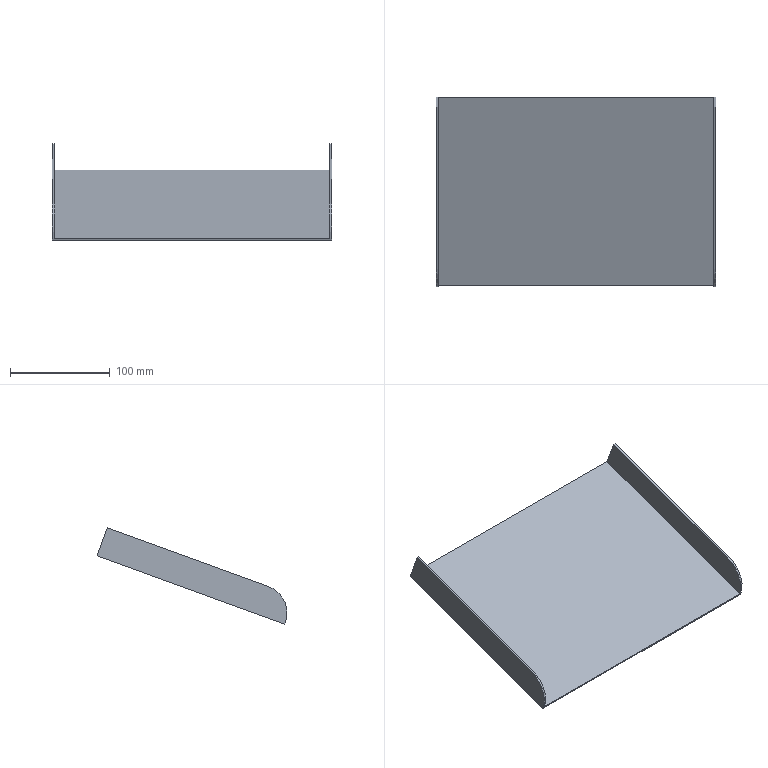Part | NX | features solid 2 | 1 solid | 12 faces | box 280.45 x 190.311 x 96.595 mm | volume 133907 mm3 | plane 10 | cylinder 2 | commonest cylinder face diameters 56 x2
STEP:
#1=CARTESIAN_POINT('',(-293.45,-997.939,-367.986));
#2=VERTEX_POINT('',#1);
#3=CARTESIAN_POINT('',(-17.,-997.939,-367.986));
#4=VERTEX_POINT('',#3);
#5=CARTESIAN_POINT('',(-283.45,-997.939,-367.986));
#6=DIRECTION('',(1.,0.,0.));
#7=VECTOR('',#6,1000.);
#8=LINE('',#5,#7);
#9=EDGE_CURVE('',#2,#4,#8,.T.);
#10=ORIENTED_EDGE('',*,*,#9,.T.);
#11=CARTESIAN_POINT('',(-17.,-810.,-299.582));
#12=VERTEX_POINT('',#11);
#13=CARTESIAN_POINT('',(-17.,-838.191,-309.843));
#14=DIRECTION('',(0.,0.9397,0.342));
#15=VECTOR('',#14,1000.);
#16=LINE('',#13,#15);
#17=EDGE_CURVE('',#4,#12,#16,.T.);
#18=ORIENTED_EDGE('',*,*,#17,.T.);
#19=CARTESIAN_POINT('',(-293.45,-810.,-299.582));
#20=VERTEX_POINT('',#19);
#21=CARTESIAN_POINT('',(-283.45,-810.,-299.582));
#22=DIRECTION('',(1.,0.,0.));
#23=VECTOR('',#22,1000.);
#24=LINE('',#21,#23);
#25=EDGE_CURVE('',#20,#12,#24,.T.);
#26=ORIENTED_EDGE('',*,*,#25,.F.);
#27=CARTESIAN_POINT('',(-293.45,-838.191,-309.843));
#28=DIRECTION('',(0.,0.9397,0.342));
#29=VECTOR('',#28,1000.);
#30=LINE('',#27,#29);
#31=EDGE_CURVE('',#2,#20,#30,.T.);
#32=ORIENTED_EDGE('',*,*,#31,.F.);
#33=EDGE_LOOP('',(#10,#18,#26,#32));
#34=FACE_BOUND('',#33,.T.);
#35=CARTESIAN_POINT('',(-283.45,-838.191,-309.843));
#36=DIRECTION('',(0.,0.342,-0.9397));
#37=DIRECTION('',(-1.,0.,0.));
#38=AXIS2_PLACEMENT_3D('',#35,#36,#37);
#39=PLANE('',#38);
#40=ADVANCED_FACE('',(#34),#39,.F.);
#41=CARTESIAN_POINT('',(-295.45,-997.254,-369.866));
#42=VERTEX_POINT('',#41);
#43=CARTESIAN_POINT('',(-15.,-997.254,-369.866));
#44=VERTEX_POINT('',#43);
#45=CARTESIAN_POINT('',(-283.45,-997.254,-369.866));
#46=DIRECTION('',(1.,0.,0.));
#47=VECTOR('',#46,1000.);
#48=LINE('',#45,#47);
#49=EDGE_CURVE('',#42,#44,#48,.T.);
#50=ORIENTED_EDGE('',*,*,#49,.T.);
#51=CARTESIAN_POINT('',(-15.,-997.939,-367.986));
#52=VERTEX_POINT('',#51);
#53=CARTESIAN_POINT('',(-15.,-997.254,-369.866));
#54=DIRECTION('',(0.,-0.342,0.9397));
#55=VECTOR('',#54,1000.);
#56=LINE('',#53,#55);
#57=EDGE_CURVE('',#44,#52,#56,.T.);
#58=ORIENTED_EDGE('',*,*,#57,.T.);
#59=CARTESIAN_POINT('',(-15.,-997.939,-367.986));
#60=DIRECTION('',(-1.,0.,0.));
#61=VECTOR('',#60,1000.);
#62=LINE('',#59,#61);
#63=EDGE_CURVE('',#52,#4,#62,.T.);
#64=ORIENTED_EDGE('',*,*,#63,.T.);
#65=ORIENTED_EDGE('',*,*,#9,.F.);
#66=CARTESIAN_POINT('',(-295.45,-997.939,-367.986));
#67=VERTEX_POINT('',#66);
#68=CARTESIAN_POINT('',(-283.45,-997.939,-367.986));
#69=DIRECTION('',(1.,0.,0.));
#70=VECTOR('',#69,1000.);
#71=LINE('',#68,#70);
#72=EDGE_CURVE('',#67,#2,#71,.T.);
#73=ORIENTED_EDGE('',*,*,#72,.F.);
#74=CARTESIAN_POINT('',(-295.45,-997.254,-369.866));
#75=DIRECTION('',(0.,-0.342,0.9397));
#76=VECTOR('',#75,1000.);
#77=LINE('',#74,#76);
#78=EDGE_CURVE('',#42,#67,#77,.T.);
#79=ORIENTED_EDGE('',*,*,#78,.F.);
#80=EDGE_LOOP('',(#50,#58,#64,#65,#73,#79));
#81=FACE_BOUND('',#80,.T.);
#82=CARTESIAN_POINT('',(-283.45,-997.254,-369.866));
#83=DIRECTION('',(0.,-0.9397,-0.342));
#84=DIRECTION('',(0.,0.342,-0.9397));
#85=AXIS2_PLACEMENT_3D('',#82,#83,#84);
#86=PLANE('',#85);
#87=ADVANCED_FACE('',(#81),#86,.T.);
#88=ORIENTED_EDGE('',*,*,#78,.T.);
#89=CARTESIAN_POINT('',(-295.45,-981.204,-332.098));
#90=VERTEX_POINT('',#89);
#91=CARTESIAN_POINT('',(-295.45,-971.627,-358.41));
#92=DIRECTION('',(-1.,0.,0.));
#93=DIRECTION('',(0.,0.,1.));
#94=AXIS2_PLACEMENT_3D('',#91,#92,#93);
#95=CIRCLE('',#94,28.);
#96=EDGE_CURVE('',#67,#90,#95,.T.);
#97=ORIENTED_EDGE('',*,*,#96,.T.);
#98=CARTESIAN_POINT('',(-295.45,-819.577,-273.271));
#99=VERTEX_POINT('',#98);
#100=CARTESIAN_POINT('',(-295.45,-819.577,-273.271));
#101=DIRECTION('',(0.,-0.9397,-0.342));
#102=VECTOR('',#101,1000.);
#103=LINE('',#100,#102);
#104=EDGE_CURVE('',#99,#90,#103,.T.);
#105=ORIENTED_EDGE('',*,*,#104,.F.);
#106=CARTESIAN_POINT('',(-295.45,-809.316,-301.462));
#107=VERTEX_POINT('',#106);
#108=CARTESIAN_POINT('',(-295.45,-809.316,-301.462));
#109=DIRECTION('',(0.,-0.342,0.9397));
#110=VECTOR('',#109,1000.);
#111=LINE('',#108,#110);
#112=EDGE_CURVE('',#107,#99,#111,.T.);
#113=ORIENTED_EDGE('',*,*,#112,.F.);
#114=CARTESIAN_POINT('',(-295.45,-837.507,-311.722));
#115=DIRECTION('',(0.,-0.9397,-0.342));
#116=VECTOR('',#115,1000.);
#117=LINE('',#114,#116);
#118=EDGE_CURVE('',#107,#42,#117,.T.);
#119=ORIENTED_EDGE('',*,*,#118,.T.);
#120=EDGE_LOOP('',(#88,#97,#105,#113,#119));
#121=FACE_BOUND('',#120,.T.);
#122=CARTESIAN_POINT('',(-295.45,-837.507,-311.722));
#123=DIRECTION('',(-1.,0.,0.));
#124=DIRECTION('',(0.,-0.342,0.9397));
#125=AXIS2_PLACEMENT_3D('',#122,#123,#124);
#126=PLANE('',#125);
#127=ADVANCED_FACE('',(#121),#126,.T.);
#128=ORIENTED_EDGE('',*,*,#25,.T.);
#129=CARTESIAN_POINT('',(-17.,-819.577,-273.271));
#130=VERTEX_POINT('',#129);
#131=CARTESIAN_POINT('',(-17.,-809.316,-301.462));
#132=DIRECTION('',(0.,-0.342,0.9397));
#133=VECTOR('',#132,1000.);
#134=LINE('',#131,#133);
#135=EDGE_CURVE('',#12,#130,#134,.T.);
#136=ORIENTED_EDGE('',*,*,#135,.T.);
#137=CARTESIAN_POINT('',(-15.,-819.577,-273.271));
#138=VERTEX_POINT('',#137);
#139=CARTESIAN_POINT('',(-15.,-819.577,-273.271));
#140=DIRECTION('',(1.,0.,0.));
#141=VECTOR('',#140,1000.);
#142=LINE('',#139,#141);
#143=EDGE_CURVE('',#138,#130,#142,.F.);
#144=ORIENTED_EDGE('',*,*,#143,.F.);
#145=CARTESIAN_POINT('',(-15.,-809.316,-301.462));
#146=VERTEX_POINT('',#145);
#147=CARTESIAN_POINT('',(-15.,-809.316,-301.462));
#148=DIRECTION('',(0.,-0.342,0.9397));
#149=VECTOR('',#148,1000.);
#150=LINE('',#147,#149);
#151=EDGE_CURVE('',#146,#138,#150,.T.);
#152=ORIENTED_EDGE('',*,*,#151,.F.);
#153=CARTESIAN_POINT('',(-283.45,-809.316,-301.462));
#154=DIRECTION('',(1.,0.,0.));
#155=VECTOR('',#154,1000.);
#156=LINE('',#153,#155);
#157=EDGE_CURVE('',#107,#146,#156,.T.);
#158=ORIENTED_EDGE('',*,*,#157,.F.);
#159=ORIENTED_EDGE('',*,*,#112,.T.);
#160=CARTESIAN_POINT('',(-293.45,-819.577,-273.271));
#161=VERTEX_POINT('',#160);
#162=CARTESIAN_POINT('',(-295.45,-819.577,-273.271));
#163=DIRECTION('',(1.,0.,0.));
#164=VECTOR('',#163,1000.);
#165=LINE('',#162,#164);
#166=EDGE_CURVE('',#99,#161,#165,.T.);
#167=ORIENTED_EDGE('',*,*,#166,.T.);
#168=CARTESIAN_POINT('',(-293.45,-809.316,-301.462));
#169=DIRECTION('',(0.,-0.342,0.9397));
#170=VECTOR('',#169,1000.);
#171=LINE('',#168,#170);
#172=EDGE_CURVE('',#20,#161,#171,.T.);
#173=ORIENTED_EDGE('',*,*,#172,.F.);
#174=EDGE_LOOP('',(#128,#136,#144,#152,#158,#159,#167,#173));
#175=FACE_BOUND('',#174,.T.);
#176=CARTESIAN_POINT('',(-283.45,-809.316,-301.462));
#177=DIRECTION('',(0.,-0.9397,-0.342));
#178=DIRECTION('',(0.,0.342,-0.9397));
#179=AXIS2_PLACEMENT_3D('',#176,#177,#178);
#180=PLANE('',#179);
#181=ADVANCED_FACE('',(#175),#180,.F.);
#182=ORIENTED_EDGE('',*,*,#151,.T.);
#183=CARTESIAN_POINT('',(-15.,-981.204,-332.098));
#184=VERTEX_POINT('',#183);
#185=CARTESIAN_POINT('',(-15.,-819.577,-273.271));
#186=DIRECTION('',(0.,-0.9397,-0.342));
#187=VECTOR('',#186,1000.);
#188=LINE('',#185,#187);
#189=EDGE_CURVE('',#138,#184,#188,.T.);
#190=ORIENTED_EDGE('',*,*,#189,.T.);
#191=CARTESIAN_POINT('',(-15.,-971.627,-358.41));
#192=DIRECTION('',(-1.,0.,0.));
#193=DIRECTION('',(0.,0.,1.));
#194=AXIS2_PLACEMENT_3D('',#191,#192,#193);
#195=CIRCLE('',#194,28.);
#196=EDGE_CURVE('',#184,#52,#195,.F.);
#197=ORIENTED_EDGE('',*,*,#196,.T.);
#198=ORIENTED_EDGE('',*,*,#57,.F.);
#199=CARTESIAN_POINT('',(-15.,-837.507,-311.722));
#200=DIRECTION('',(0.,-0.9397,-0.342));
#201=VECTOR('',#200,1000.);
#202=LINE('',#199,#201);
#203=EDGE_CURVE('',#146,#44,#202,.T.);
#204=ORIENTED_EDGE('',*,*,#203,.F.);
#205=EDGE_LOOP('',(#182,#190,#197,#198,#204));
#206=FACE_BOUND('',#205,.T.);
#207=CARTESIAN_POINT('',(-15.,-837.507,-311.722));
#208=DIRECTION('',(-1.,0.,0.));
#209=DIRECTION('',(0.,-0.342,0.9397));
#210=AXIS2_PLACEMENT_3D('',#207,#208,#209);
#211=PLANE('',#210);
#212=ADVANCED_FACE('',(#206),#211,.F.);
#213=ORIENTED_EDGE('',*,*,#157,.T.);
#214=ORIENTED_EDGE('',*,*,#203,.T.);
#215=ORIENTED_EDGE('',*,*,#49,.F.);
#216=ORIENTED_EDGE('',*,*,#118,.F.);
#217=EDGE_LOOP('',(#213,#214,#215,#216));
#218=FACE_BOUND('',#217,.T.);
#219=CARTESIAN_POINT('',(-283.45,-837.507,-311.722));
#220=DIRECTION('',(0.,0.342,-0.9397));
#221=DIRECTION('',(-1.,0.,0.));
#222=AXIS2_PLACEMENT_3D('',#219,#220,#221);
#223=PLANE('',#222);
#224=ADVANCED_FACE('',(#218),#223,.T.);
#225=CARTESIAN_POINT('',(-293.45,-981.204,-332.098));
#226=VERTEX_POINT('',#225);
#227=CARTESIAN_POINT('',(-293.45,-971.627,-358.41));
#228=DIRECTION('',(-1.,0.,0.));
#229=DIRECTION('',(0.,0.,1.));
#230=AXIS2_PLACEMENT_3D('',#227,#228,#229);
#231=CIRCLE('',#230,28.);
#232=EDGE_CURVE('',#226,#2,#231,.F.);
#233=ORIENTED_EDGE('',*,*,#232,.T.);
#234=ORIENTED_EDGE('',*,*,#31,.T.);
#235=ORIENTED_EDGE('',*,*,#172,.T.);
#236=CARTESIAN_POINT('',(-293.45,-819.577,-273.271));
#237=DIRECTION('',(0.,-0.9397,-0.342));
#238=VECTOR('',#237,1000.);
#239=LINE('',#236,#238);
#240=EDGE_CURVE('',#161,#226,#239,.T.);
#241=ORIENTED_EDGE('',*,*,#240,.T.);
#242=EDGE_LOOP('',(#233,#234,#235,#241));
#243=FACE_BOUND('',#242,.T.);
#244=CARTESIAN_POINT('',(-293.45,-809.316,-301.462));
#245=DIRECTION('',(-1.,0.,0.));
#246=DIRECTION('',(0.,0.,1.));
#247=AXIS2_PLACEMENT_3D('',#244,#245,#246);
#248=PLANE('',#247);
#249=ADVANCED_FACE('',(#243),#248,.F.);
#250=ORIENTED_EDGE('',*,*,#104,.T.);
#251=CARTESIAN_POINT('',(-295.45,-981.204,-332.098));
#252=DIRECTION('',(1.,0.,0.));
#253=VECTOR('',#252,1000.);
#254=LINE('',#251,#253);
#255=EDGE_CURVE('',#90,#226,#254,.T.);
#256=ORIENTED_EDGE('',*,*,#255,.T.);
#257=ORIENTED_EDGE('',*,*,#240,.F.);
#258=ORIENTED_EDGE('',*,*,#166,.F.);
#259=EDGE_LOOP('',(#250,#256,#257,#258));
#260=FACE_BOUND('',#259,.T.);
#261=CARTESIAN_POINT('',(-295.45,-819.577,-273.271));
#262=DIRECTION('',(0.,0.342,-0.9397));
#263=DIRECTION('',(0.,-0.9397,-0.342));
#264=AXIS2_PLACEMENT_3D('',#261,#262,#263);
#265=PLANE('',#264);
#266=ADVANCED_FACE('',(#260),#265,.F.);
#267=ORIENTED_EDGE('',*,*,#96,.F.);
#268=ORIENTED_EDGE('',*,*,#72,.T.);
#269=ORIENTED_EDGE('',*,*,#232,.F.);
#270=ORIENTED_EDGE('',*,*,#255,.F.);
#271=EDGE_LOOP('',(#267,#268,#269,#270));
#272=FACE_BOUND('',#271,.T.);
#273=CARTESIAN_POINT('',(-295.45,-971.627,-358.41));
#274=DIRECTION('',(-1.,0.,0.));
#275=DIRECTION('',(0.,0.,1.));
#276=AXIS2_PLACEMENT_3D('',#273,#274,#275);
#277=CYLINDRICAL_SURFACE('',#276,28.);
#278=ADVANCED_FACE('',(#272),#277,.T.);
#279=ORIENTED_EDGE('',*,*,#17,.F.);
#280=CARTESIAN_POINT('',(-17.,-981.204,-332.098));
#281=VERTEX_POINT('',#280);
#282=CARTESIAN_POINT('',(-17.,-971.627,-358.41));
#283=DIRECTION('',(-1.,0.,0.));
#284=DIRECTION('',(0.,0.,1.));
#285=AXIS2_PLACEMENT_3D('',#282,#283,#284);
#286=CIRCLE('',#285,28.);
#287=EDGE_CURVE('',#4,#281,#286,.T.);
#288=ORIENTED_EDGE('',*,*,#287,.T.);
#289=CARTESIAN_POINT('',(-17.,-819.577,-273.271));
#290=DIRECTION('',(0.,-0.9397,-0.342));
#291=VECTOR('',#290,1000.);
#292=LINE('',#289,#291);
#293=EDGE_CURVE('',#130,#281,#292,.T.);
#294=ORIENTED_EDGE('',*,*,#293,.F.);
#295=ORIENTED_EDGE('',*,*,#135,.F.);
#296=EDGE_LOOP('',(#279,#288,#294,#295));
#297=FACE_BOUND('',#296,.T.);
#298=CARTESIAN_POINT('',(-17.,-809.316,-301.462));
#299=DIRECTION('',(-1.,0.,0.));
#300=DIRECTION('',(0.,0.,1.));
#301=AXIS2_PLACEMENT_3D('',#298,#299,#300);
#302=PLANE('',#301);
#303=ADVANCED_FACE('',(#297),#302,.T.);
#304=ORIENTED_EDGE('',*,*,#293,.T.);
#305=CARTESIAN_POINT('',(-15.,-981.204,-332.098));
#306=DIRECTION('',(1.,0.,0.));
#307=VECTOR('',#306,1000.);
#308=LINE('',#305,#307);
#309=EDGE_CURVE('',#281,#184,#308,.T.);
#310=ORIENTED_EDGE('',*,*,#309,.T.);
#311=ORIENTED_EDGE('',*,*,#189,.F.);
#312=ORIENTED_EDGE('',*,*,#143,.T.);
#313=EDGE_LOOP('',(#304,#310,#311,#312));
#314=FACE_BOUND('',#313,.T.);
#315=CARTESIAN_POINT('',(-15.,-819.577,-273.271));
#316=DIRECTION('',(0.,0.342,-0.9397));
#317=DIRECTION('',(0.,-0.9397,-0.342));
#318=AXIS2_PLACEMENT_3D('',#315,#316,#317);
#319=PLANE('',#318);
#320=ADVANCED_FACE('',(#314),#319,.F.);
#321=ORIENTED_EDGE('',*,*,#196,.F.);
#322=ORIENTED_EDGE('',*,*,#309,.F.);
#323=ORIENTED_EDGE('',*,*,#287,.F.);
#324=ORIENTED_EDGE('',*,*,#63,.F.);
#325=EDGE_LOOP('',(#321,#322,#323,#324));
#326=FACE_BOUND('',#325,.T.);
#327=CARTESIAN_POINT('',(-15.,-971.627,-358.41));
#328=DIRECTION('',(1.,0.,0.));
#329=DIRECTION('',(0.,0.,-1.));
#330=AXIS2_PLACEMENT_3D('',#327,#328,#329);
#331=CYLINDRICAL_SURFACE('',#330,28.);
#332=ADVANCED_FACE('',(#326),#331,.T.);
#333=CLOSED_SHELL('',(#40,#87,#127,#181,#212,#224,#249,#266,#278,#303,#320,#332));
#334=MANIFOLD_SOLID_BREP('',#333);
#335=(LENGTH_UNIT()NAMED_UNIT(*)SI_UNIT(.MILLI.,.METRE.));
#336=UNCERTAINTY_MEASURE_WITH_UNIT(LENGTH_MEASURE(0.00001),#335,'','');
#337=(NAMED_UNIT(*)PLANE_ANGLE_UNIT()SI_UNIT($,.RADIAN.));
#338=(NAMED_UNIT(*)SI_UNIT($,.STERADIAN.)SOLID_ANGLE_UNIT());
#339=(GEOMETRIC_REPRESENTATION_CONTEXT(3)GLOBAL_UNCERTAINTY_ASSIGNED_CONTEXT((#336))GLOBAL_UNIT_ASSIGNED_CONTEXT((#335,#337,#338))REPRESENTATION_CONTEXT('',''));
#340=ADVANCED_BREP_SHAPE_REPRESENTATION('',(#334),#339);